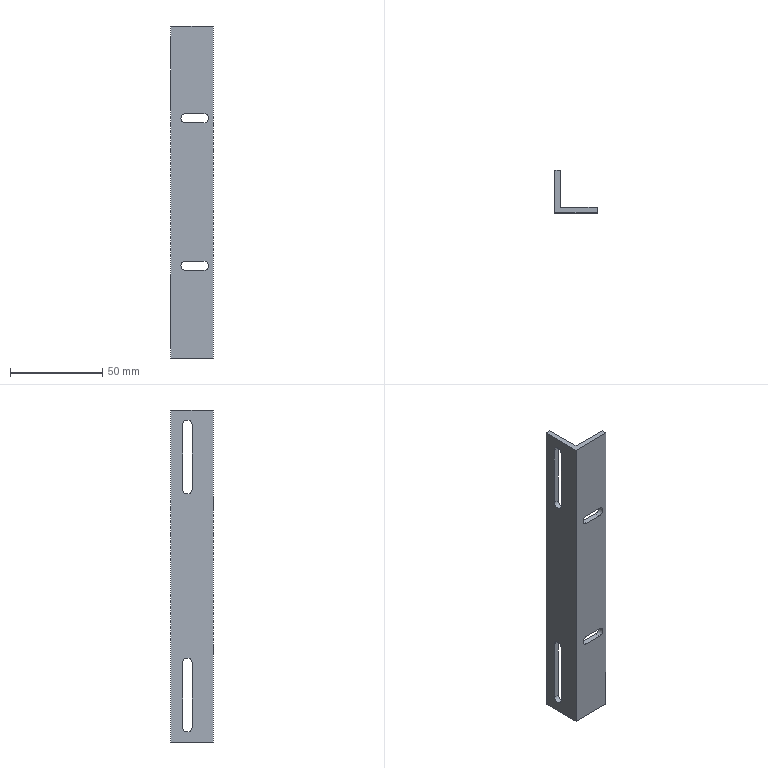Part | SolidWorks | features ICE 2, Extrusion 1, MirrorPattern 1 | 1 solid | 26 faces | box 23 x 23 x 180 mm | volume 21634 mm3 | plane 16 | cylinder 10 | commonest cylinder face diameters 5 x10
STEP:
#1=CARTESIAN_POINT('',(8.,0.,-37.5));
#2=VERTEX_POINT('',#1);
#3=CARTESIAN_POINT('',(5.5,0.,-40.));
#4=VERTEX_POINT('',#3);
#5=CARTESIAN_POINT('',(8.,0.,-40.));
#6=DIRECTION('',(0.,-1.,0.));
#7=DIRECTION('',(-1.,0.,0.));
#8=AXIS2_PLACEMENT_3D('',#5,#6,#7);
#9=CIRCLE('',#8,2.5);
#10=EDGE_CURVE('',#2,#4,#9,.T.);
#11=ORIENTED_EDGE('',*,*,#10,.T.);
#12=CARTESIAN_POINT('',(5.5,3.,-40.));
#13=VERTEX_POINT('',#12);
#14=CARTESIAN_POINT('',(5.5,-0.001,-40.));
#15=DIRECTION('',(0.,1.,0.));
#16=VECTOR('',#15,1000.);
#17=LINE('',#14,#16);
#18=EDGE_CURVE('',#4,#13,#17,.T.);
#19=ORIENTED_EDGE('',*,*,#18,.T.);
#20=CARTESIAN_POINT('',(8.,3.,-37.5));
#21=VERTEX_POINT('',#20);
#22=CARTESIAN_POINT('',(8.,3.,-40.));
#23=DIRECTION('',(0.,1.,0.));
#24=DIRECTION('',(-1.,0.,0.));
#25=AXIS2_PLACEMENT_3D('',#22,#23,#24);
#26=CIRCLE('',#25,2.5);
#27=EDGE_CURVE('',#13,#21,#26,.T.);
#28=ORIENTED_EDGE('',*,*,#27,.T.);
#29=CARTESIAN_POINT('',(8.,-0.001,-37.5));
#30=DIRECTION('',(0.,1.,0.));
#31=VECTOR('',#30,1000.);
#32=LINE('',#29,#31);
#33=EDGE_CURVE('',#2,#21,#32,.T.);
#34=ORIENTED_EDGE('',*,*,#33,.F.);
#35=EDGE_LOOP('',(#11,#19,#28,#34));
#36=FACE_OUTER_BOUND('',#35,.T.);
#37=CARTESIAN_POINT('',(8.,-0.001,-40.));
#38=DIRECTION('',(0.,1.,0.));
#39=DIRECTION('',(-1.,0.,0.));
#40=AXIS2_PLACEMENT_3D('',#37,#38,#39);
#41=CYLINDRICAL_SURFACE('',#40,2.5);
#42=ADVANCED_FACE('',(#36),#41,.F.);
#43=CARTESIAN_POINT('',(8.,0.,42.5));
#44=VERTEX_POINT('',#43);
#45=CARTESIAN_POINT('',(5.5,0.,40.));
#46=VERTEX_POINT('',#45);
#47=CARTESIAN_POINT('',(8.,0.,40.));
#48=DIRECTION('',(0.,-1.,0.));
#49=DIRECTION('',(-1.,0.,0.));
#50=AXIS2_PLACEMENT_3D('',#47,#48,#49);
#51=CIRCLE('',#50,2.5);
#52=EDGE_CURVE('',#44,#46,#51,.T.);
#53=ORIENTED_EDGE('',*,*,#52,.T.);
#54=CARTESIAN_POINT('',(5.5,3.,40.));
#55=VERTEX_POINT('',#54);
#56=CARTESIAN_POINT('',(5.5,-0.001,40.));
#57=DIRECTION('',(0.,1.,0.));
#58=VECTOR('',#57,1000.);
#59=LINE('',#56,#58);
#60=EDGE_CURVE('',#46,#55,#59,.T.);
#61=ORIENTED_EDGE('',*,*,#60,.T.);
#62=CARTESIAN_POINT('',(8.,3.,42.5));
#63=VERTEX_POINT('',#62);
#64=CARTESIAN_POINT('',(8.,3.,40.));
#65=DIRECTION('',(0.,1.,0.));
#66=DIRECTION('',(-1.,0.,0.));
#67=AXIS2_PLACEMENT_3D('',#64,#65,#66);
#68=CIRCLE('',#67,2.5);
#69=EDGE_CURVE('',#55,#63,#68,.T.);
#70=ORIENTED_EDGE('',*,*,#69,.T.);
#71=CARTESIAN_POINT('',(8.,-0.001,42.5));
#72=DIRECTION('',(0.,1.,0.));
#73=VECTOR('',#72,1000.);
#74=LINE('',#71,#73);
#75=EDGE_CURVE('',#44,#63,#74,.T.);
#76=ORIENTED_EDGE('',*,*,#75,.F.);
#77=EDGE_LOOP('',(#53,#61,#70,#76));
#78=FACE_OUTER_BOUND('',#77,.T.);
#79=CARTESIAN_POINT('',(8.,-0.001,40.));
#80=DIRECTION('',(0.,1.,0.));
#81=DIRECTION('',(-1.,0.,0.));
#82=AXIS2_PLACEMENT_3D('',#79,#80,#81);
#83=CYLINDRICAL_SURFACE('',#82,2.5);
#84=ADVANCED_FACE('',(#78),#83,.F.);
#85=CARTESIAN_POINT('',(3.,3.,-90.));
#86=VERTEX_POINT('',#85);
#87=CARTESIAN_POINT('',(3.,23.,-90.));
#88=VERTEX_POINT('',#87);
#89=CARTESIAN_POINT('',(3.,23.,-90.));
#90=DIRECTION('',(0.,1.,0.));
#91=VECTOR('',#90,1000.);
#92=LINE('',#89,#91);
#93=EDGE_CURVE('',#86,#88,#92,.T.);
#94=ORIENTED_EDGE('',*,*,#93,.T.);
#95=CARTESIAN_POINT('',(3.,23.,90.));
#96=VERTEX_POINT('',#95);
#97=CARTESIAN_POINT('',(3.,23.,90.));
#98=DIRECTION('',(0.,0.,-1.));
#99=VECTOR('',#98,1000.);
#100=LINE('',#97,#99);
#101=EDGE_CURVE('',#96,#88,#100,.T.);
#102=ORIENTED_EDGE('',*,*,#101,.F.);
#103=CARTESIAN_POINT('',(3.,3.,90.));
#104=VERTEX_POINT('',#103);
#105=CARTESIAN_POINT('',(3.,23.,90.));
#106=DIRECTION('',(0.,1.,0.));
#107=VECTOR('',#106,1000.);
#108=LINE('',#105,#107);
#109=EDGE_CURVE('',#104,#96,#108,.T.);
#110=ORIENTED_EDGE('',*,*,#109,.F.);
#111=CARTESIAN_POINT('',(3.,3.,90.));
#112=DIRECTION('',(0.,0.,-1.));
#113=VECTOR('',#112,1000.);
#114=LINE('',#111,#113);
#115=EDGE_CURVE('',#104,#86,#114,.T.);
#116=ORIENTED_EDGE('',*,*,#115,.T.);
#117=EDGE_LOOP('',(#94,#102,#110,#116));
#118=FACE_OUTER_BOUND('',#117,.T.);
#119=CARTESIAN_POINT('',(3.,11.5,82.));
#120=VERTEX_POINT('',#119);
#121=CARTESIAN_POINT('',(3.,11.5,47.));
#122=VERTEX_POINT('',#121);
#123=CARTESIAN_POINT('',(3.,11.5,82.));
#124=DIRECTION('',(0.,0.,-1.));
#125=VECTOR('',#124,1000.);
#126=LINE('',#123,#125);
#127=EDGE_CURVE('',#120,#122,#126,.T.);
#128=ORIENTED_EDGE('',*,*,#127,.F.);
#129=CARTESIAN_POINT('',(3.,16.5,82.));
#130=VERTEX_POINT('',#129);
#131=CARTESIAN_POINT('',(3.,14.,82.));
#132=DIRECTION('',(1.,0.,0.));
#133=DIRECTION('',(0.,1.,0.));
#134=AXIS2_PLACEMENT_3D('',#131,#132,#133);
#135=CIRCLE('',#134,2.5);
#136=EDGE_CURVE('',#130,#120,#135,.T.);
#137=ORIENTED_EDGE('',*,*,#136,.F.);
#138=CARTESIAN_POINT('',(3.,16.5,47.));
#139=VERTEX_POINT('',#138);
#140=CARTESIAN_POINT('',(3.,16.5,82.));
#141=DIRECTION('',(0.,0.,1.));
#142=VECTOR('',#141,1000.);
#143=LINE('',#140,#142);
#144=EDGE_CURVE('',#139,#130,#143,.T.);
#145=ORIENTED_EDGE('',*,*,#144,.F.);
#146=CARTESIAN_POINT('',(3.,14.,47.));
#147=DIRECTION('',(1.,0.,0.));
#148=DIRECTION('',(0.,1.,0.));
#149=AXIS2_PLACEMENT_3D('',#146,#147,#148);
#150=CIRCLE('',#149,2.5);
#151=EDGE_CURVE('',#122,#139,#150,.T.);
#152=ORIENTED_EDGE('',*,*,#151,.F.);
#153=EDGE_LOOP('',(#128,#137,#145,#152));
#154=FACE_BOUND('',#153,.T.);
#155=CARTESIAN_POINT('',(3.,16.5,-82.));
#156=VERTEX_POINT('',#155);
#157=CARTESIAN_POINT('',(3.,11.5,-82.));
#158=VERTEX_POINT('',#157);
#159=CARTESIAN_POINT('',(3.,14.,-82.));
#160=DIRECTION('',(-1.,0.,0.));
#161=DIRECTION('',(0.,1.,0.));
#162=AXIS2_PLACEMENT_3D('',#159,#160,#161);
#163=CIRCLE('',#162,2.5);
#164=EDGE_CURVE('',#156,#158,#163,.T.);
#165=ORIENTED_EDGE('',*,*,#164,.T.);
#166=CARTESIAN_POINT('',(3.,11.5,-47.));
#167=VERTEX_POINT('',#166);
#168=CARTESIAN_POINT('',(3.,11.5,-82.));
#169=DIRECTION('',(0.,0.,1.));
#170=VECTOR('',#169,1000.);
#171=LINE('',#168,#170);
#172=EDGE_CURVE('',#158,#167,#171,.T.);
#173=ORIENTED_EDGE('',*,*,#172,.T.);
#174=CARTESIAN_POINT('',(3.,16.5,-47.));
#175=VERTEX_POINT('',#174);
#176=CARTESIAN_POINT('',(3.,14.,-47.));
#177=DIRECTION('',(-1.,0.,0.));
#178=DIRECTION('',(0.,1.,0.));
#179=AXIS2_PLACEMENT_3D('',#176,#177,#178);
#180=CIRCLE('',#179,2.5);
#181=EDGE_CURVE('',#167,#175,#180,.T.);
#182=ORIENTED_EDGE('',*,*,#181,.T.);
#183=CARTESIAN_POINT('',(3.,16.5,-82.));
#184=DIRECTION('',(0.,0.,-1.));
#185=VECTOR('',#184,1000.);
#186=LINE('',#183,#185);
#187=EDGE_CURVE('',#175,#156,#186,.T.);
#188=ORIENTED_EDGE('',*,*,#187,.T.);
#189=EDGE_LOOP('',(#165,#173,#182,#188));
#190=FACE_BOUND('',#189,.T.);
#191=CARTESIAN_POINT('',(3.,23.,90.));
#192=DIRECTION('',(-1.,0.,0.));
#193=DIRECTION('',(0.,-1.,0.));
#194=AXIS2_PLACEMENT_3D('',#191,#192,#193);
#195=PLANE('',#194);
#196=ADVANCED_FACE('',(#118,#154,#190),#195,.F.);
#197=CARTESIAN_POINT('',(0.,23.,-90.));
#198=VERTEX_POINT('',#197);
#199=CARTESIAN_POINT('',(0.,0.,-90.));
#200=VERTEX_POINT('',#199);
#201=CARTESIAN_POINT('',(0.,0.,-90.));
#202=DIRECTION('',(0.,-1.,0.));
#203=VECTOR('',#202,1000.);
#204=LINE('',#201,#203);
#205=EDGE_CURVE('',#198,#200,#204,.T.);
#206=ORIENTED_EDGE('',*,*,#205,.T.);
#207=CARTESIAN_POINT('',(0.,0.,90.));
#208=VERTEX_POINT('',#207);
#209=CARTESIAN_POINT('',(0.,0.,90.));
#210=DIRECTION('',(0.,0.,-1.));
#211=VECTOR('',#210,1000.);
#212=LINE('',#209,#211);
#213=EDGE_CURVE('',#208,#200,#212,.T.);
#214=ORIENTED_EDGE('',*,*,#213,.F.);
#215=CARTESIAN_POINT('',(0.,23.,90.));
#216=VERTEX_POINT('',#215);
#217=CARTESIAN_POINT('',(0.,0.,90.));
#218=DIRECTION('',(0.,-1.,0.));
#219=VECTOR('',#218,1000.);
#220=LINE('',#217,#219);
#221=EDGE_CURVE('',#216,#208,#220,.T.);
#222=ORIENTED_EDGE('',*,*,#221,.F.);
#223=CARTESIAN_POINT('',(0.,23.,90.));
#224=DIRECTION('',(0.,0.,-1.));
#225=VECTOR('',#224,1000.);
#226=LINE('',#223,#225);
#227=EDGE_CURVE('',#216,#198,#226,.T.);
#228=ORIENTED_EDGE('',*,*,#227,.T.);
#229=EDGE_LOOP('',(#206,#214,#222,#228));
#230=FACE_OUTER_BOUND('',#229,.T.);
#231=CARTESIAN_POINT('',(0.,16.5,82.));
#232=VERTEX_POINT('',#231);
#233=CARTESIAN_POINT('',(0.,16.5,47.));
#234=VERTEX_POINT('',#233);
#235=CARTESIAN_POINT('',(0.,16.5,82.));
#236=DIRECTION('',(0.,0.,-1.));
#237=VECTOR('',#236,1000.);
#238=LINE('',#235,#237);
#239=EDGE_CURVE('',#232,#234,#238,.T.);
#240=ORIENTED_EDGE('',*,*,#239,.F.);
#241=CARTESIAN_POINT('',(0.,11.5,82.));
#242=VERTEX_POINT('',#241);
#243=CARTESIAN_POINT('',(0.,14.,82.));
#244=DIRECTION('',(-1.,0.,0.));
#245=DIRECTION('',(0.,1.,0.));
#246=AXIS2_PLACEMENT_3D('',#243,#244,#245);
#247=CIRCLE('',#246,2.5);
#248=EDGE_CURVE('',#242,#232,#247,.T.);
#249=ORIENTED_EDGE('',*,*,#248,.F.);
#250=CARTESIAN_POINT('',(0.,11.5,47.));
#251=VERTEX_POINT('',#250);
#252=CARTESIAN_POINT('',(0.,11.5,82.));
#253=DIRECTION('',(0.,0.,1.));
#254=VECTOR('',#253,1000.);
#255=LINE('',#252,#254);
#256=EDGE_CURVE('',#251,#242,#255,.T.);
#257=ORIENTED_EDGE('',*,*,#256,.F.);
#258=CARTESIAN_POINT('',(0.,14.,47.));
#259=DIRECTION('',(-1.,0.,0.));
#260=DIRECTION('',(0.,1.,0.));
#261=AXIS2_PLACEMENT_3D('',#258,#259,#260);
#262=CIRCLE('',#261,2.5);
#263=EDGE_CURVE('',#234,#251,#262,.T.);
#264=ORIENTED_EDGE('',*,*,#263,.F.);
#265=EDGE_LOOP('',(#240,#249,#257,#264));
#266=FACE_BOUND('',#265,.T.);
#267=CARTESIAN_POINT('',(0.,11.5,-82.));
#268=VERTEX_POINT('',#267);
#269=CARTESIAN_POINT('',(0.,16.5,-82.));
#270=VERTEX_POINT('',#269);
#271=CARTESIAN_POINT('',(0.,14.,-82.));
#272=DIRECTION('',(1.,0.,0.));
#273=DIRECTION('',(0.,1.,0.));
#274=AXIS2_PLACEMENT_3D('',#271,#272,#273);
#275=CIRCLE('',#274,2.5);
#276=EDGE_CURVE('',#268,#270,#275,.T.);
#277=ORIENTED_EDGE('',*,*,#276,.T.);
#278=CARTESIAN_POINT('',(0.,16.5,-47.));
#279=VERTEX_POINT('',#278);
#280=CARTESIAN_POINT('',(0.,16.5,-82.));
#281=DIRECTION('',(0.,0.,1.));
#282=VECTOR('',#281,1000.);
#283=LINE('',#280,#282);
#284=EDGE_CURVE('',#270,#279,#283,.T.);
#285=ORIENTED_EDGE('',*,*,#284,.T.);
#286=CARTESIAN_POINT('',(0.,11.5,-47.));
#287=VERTEX_POINT('',#286);
#288=CARTESIAN_POINT('',(0.,14.,-47.));
#289=DIRECTION('',(1.,0.,0.));
#290=DIRECTION('',(0.,1.,0.));
#291=AXIS2_PLACEMENT_3D('',#288,#289,#290);
#292=CIRCLE('',#291,2.5);
#293=EDGE_CURVE('',#279,#287,#292,.T.);
#294=ORIENTED_EDGE('',*,*,#293,.T.);
#295=CARTESIAN_POINT('',(0.,11.5,-82.));
#296=DIRECTION('',(0.,0.,-1.));
#297=VECTOR('',#296,1000.);
#298=LINE('',#295,#297);
#299=EDGE_CURVE('',#287,#268,#298,.T.);
#300=ORIENTED_EDGE('',*,*,#299,.T.);
#301=EDGE_LOOP('',(#277,#285,#294,#300));
#302=FACE_BOUND('',#301,.T.);
#303=CARTESIAN_POINT('',(0.,0.,90.));
#304=DIRECTION('',(1.,0.,0.));
#305=DIRECTION('',(0.,1.,0.));
#306=AXIS2_PLACEMENT_3D('',#303,#304,#305);
#307=PLANE('',#306);
#308=ADVANCED_FACE('',(#230,#266,#302),#307,.F.);
#309=CARTESIAN_POINT('',(8.,0.,-42.5));
#310=VERTEX_POINT('',#309);
#311=CARTESIAN_POINT('',(18.,0.,-42.5));
#312=VERTEX_POINT('',#311);
#313=CARTESIAN_POINT('',(8.,0.,-42.5));
#314=DIRECTION('',(1.,0.,0.));
#315=VECTOR('',#314,1000.);
#316=LINE('',#313,#315);
#317=EDGE_CURVE('',#310,#312,#316,.T.);
#318=ORIENTED_EDGE('',*,*,#317,.F.);
#319=CARTESIAN_POINT('',(8.,0.,-40.));
#320=DIRECTION('',(0.,-1.,0.));
#321=DIRECTION('',(-1.,0.,0.));
#322=AXIS2_PLACEMENT_3D('',#319,#320,#321);
#323=CIRCLE('',#322,2.5);
#324=EDGE_CURVE('',#4,#310,#323,.T.);
#325=ORIENTED_EDGE('',*,*,#324,.F.);
#326=ORIENTED_EDGE('',*,*,#10,.F.);
#327=CARTESIAN_POINT('',(18.,0.,-37.5));
#328=VERTEX_POINT('',#327);
#329=CARTESIAN_POINT('',(8.,0.,-37.5));
#330=DIRECTION('',(-1.,0.,0.));
#331=VECTOR('',#330,1000.);
#332=LINE('',#329,#331);
#333=EDGE_CURVE('',#328,#2,#332,.T.);
#334=ORIENTED_EDGE('',*,*,#333,.F.);
#335=CARTESIAN_POINT('',(18.,0.,-40.));
#336=DIRECTION('',(0.,-1.,0.));
#337=DIRECTION('',(-1.,0.,0.));
#338=AXIS2_PLACEMENT_3D('',#335,#336,#337);
#339=CIRCLE('',#338,2.5);
#340=EDGE_CURVE('',#312,#328,#339,.T.);
#341=ORIENTED_EDGE('',*,*,#340,.F.);
#342=EDGE_LOOP('',(#318,#325,#326,#334,#341));
#343=FACE_BOUND('',#342,.T.);
#344=CARTESIAN_POINT('',(8.,0.,37.5));
#345=VERTEX_POINT('',#344);
#346=CARTESIAN_POINT('',(18.,0.,37.5));
#347=VERTEX_POINT('',#346);
#348=CARTESIAN_POINT('',(8.,0.,37.5));
#349=DIRECTION('',(1.,0.,0.));
#350=VECTOR('',#349,1000.);
#351=LINE('',#348,#350);
#352=EDGE_CURVE('',#345,#347,#351,.T.);
#353=ORIENTED_EDGE('',*,*,#352,.F.);
#354=CARTESIAN_POINT('',(8.,0.,40.));
#355=DIRECTION('',(0.,-1.,0.));
#356=DIRECTION('',(-1.,0.,0.));
#357=AXIS2_PLACEMENT_3D('',#354,#355,#356);
#358=CIRCLE('',#357,2.5);
#359=EDGE_CURVE('',#46,#345,#358,.T.);
#360=ORIENTED_EDGE('',*,*,#359,.F.);
#361=ORIENTED_EDGE('',*,*,#52,.F.);
#362=CARTESIAN_POINT('',(18.,0.,42.5));
#363=VERTEX_POINT('',#362);
#364=CARTESIAN_POINT('',(8.,0.,42.5));
#365=DIRECTION('',(-1.,0.,0.));
#366=VECTOR('',#365,1000.);
#367=LINE('',#364,#366);
#368=EDGE_CURVE('',#363,#44,#367,.T.);
#369=ORIENTED_EDGE('',*,*,#368,.F.);
#370=CARTESIAN_POINT('',(18.,0.,40.));
#371=DIRECTION('',(0.,-1.,0.));
#372=DIRECTION('',(-1.,0.,0.));
#373=AXIS2_PLACEMENT_3D('',#370,#371,#372);
#374=CIRCLE('',#373,2.5);
#375=EDGE_CURVE('',#347,#363,#374,.T.);
#376=ORIENTED_EDGE('',*,*,#375,.F.);
#377=EDGE_LOOP('',(#353,#360,#361,#369,#376));
#378=FACE_BOUND('',#377,.T.);
#379=CARTESIAN_POINT('',(23.,0.,-90.));
#380=VERTEX_POINT('',#379);
#381=CARTESIAN_POINT('',(23.,0.,-90.));
#382=DIRECTION('',(1.,0.,0.));
#383=VECTOR('',#382,1000.);
#384=LINE('',#381,#383);
#385=EDGE_CURVE('',#200,#380,#384,.T.);
#386=ORIENTED_EDGE('',*,*,#385,.T.);
#387=CARTESIAN_POINT('',(23.,0.,90.));
#388=VERTEX_POINT('',#387);
#389=CARTESIAN_POINT('',(23.,0.,90.));
#390=DIRECTION('',(0.,0.,-1.));
#391=VECTOR('',#390,1000.);
#392=LINE('',#389,#391);
#393=EDGE_CURVE('',#388,#380,#392,.T.);
#394=ORIENTED_EDGE('',*,*,#393,.F.);
#395=CARTESIAN_POINT('',(23.,0.,90.));
#396=DIRECTION('',(1.,0.,0.));
#397=VECTOR('',#396,1000.);
#398=LINE('',#395,#397);
#399=EDGE_CURVE('',#208,#388,#398,.T.);
#400=ORIENTED_EDGE('',*,*,#399,.F.);
#401=ORIENTED_EDGE('',*,*,#213,.T.);
#402=EDGE_LOOP('',(#386,#394,#400,#401));
#403=FACE_OUTER_BOUND('',#402,.T.);
#404=CARTESIAN_POINT('',(23.,0.,90.));
#405=DIRECTION('',(0.,1.,0.));
#406=DIRECTION('',(-1.,0.,0.));
#407=AXIS2_PLACEMENT_3D('',#404,#405,#406);
#408=PLANE('',#407);
#409=ADVANCED_FACE('',(#343,#378,#403),#408,.F.);
#410=CARTESIAN_POINT('',(23.,3.,-90.));
#411=VERTEX_POINT('',#410);
#412=CARTESIAN_POINT('',(23.,3.,-90.));
#413=DIRECTION('',(0.,1.,0.));
#414=VECTOR('',#413,1000.);
#415=LINE('',#412,#414);
#416=EDGE_CURVE('',#380,#411,#415,.T.);
#417=ORIENTED_EDGE('',*,*,#416,.T.);
#418=CARTESIAN_POINT('',(23.,3.,90.));
#419=VERTEX_POINT('',#418);
#420=CARTESIAN_POINT('',(23.,3.,90.));
#421=DIRECTION('',(0.,0.,-1.));
#422=VECTOR('',#421,1000.);
#423=LINE('',#420,#422);
#424=EDGE_CURVE('',#419,#411,#423,.T.);
#425=ORIENTED_EDGE('',*,*,#424,.F.);
#426=CARTESIAN_POINT('',(23.,3.,90.));
#427=DIRECTION('',(0.,1.,0.));
#428=VECTOR('',#427,1000.);
#429=LINE('',#426,#428);
#430=EDGE_CURVE('',#388,#419,#429,.T.);
#431=ORIENTED_EDGE('',*,*,#430,.F.);
#432=ORIENTED_EDGE('',*,*,#393,.T.);
#433=EDGE_LOOP('',(#417,#425,#431,#432));
#434=FACE_OUTER_BOUND('',#433,.T.);
#435=CARTESIAN_POINT('',(23.,3.,90.));
#436=DIRECTION('',(-1.,0.,0.));
#437=DIRECTION('',(0.,0.,1.));
#438=AXIS2_PLACEMENT_3D('',#435,#436,#437);
#439=PLANE('',#438);
#440=ADVANCED_FACE('',(#434),#439,.F.);
#441=CARTESIAN_POINT('',(18.,3.,-37.5));
#442=VERTEX_POINT('',#441);
#443=CARTESIAN_POINT('',(8.,3.,-37.5));
#444=DIRECTION('',(1.,0.,0.));
#445=VECTOR('',#444,1000.);
#446=LINE('',#443,#445);
#447=EDGE_CURVE('',#21,#442,#446,.T.);
#448=ORIENTED_EDGE('',*,*,#447,.F.);
#449=ORIENTED_EDGE('',*,*,#27,.F.);
#450=CARTESIAN_POINT('',(8.,3.,-42.5));
#451=VERTEX_POINT('',#450);
#452=CARTESIAN_POINT('',(8.,3.,-40.));
#453=DIRECTION('',(0.,1.,0.));
#454=DIRECTION('',(-1.,0.,0.));
#455=AXIS2_PLACEMENT_3D('',#452,#453,#454);
#456=CIRCLE('',#455,2.5);
#457=EDGE_CURVE('',#451,#13,#456,.T.);
#458=ORIENTED_EDGE('',*,*,#457,.F.);
#459=CARTESIAN_POINT('',(18.,3.,-42.5));
#460=VERTEX_POINT('',#459);
#461=CARTESIAN_POINT('',(8.,3.,-42.5));
#462=DIRECTION('',(-1.,0.,0.));
#463=VECTOR('',#462,1000.);
#464=LINE('',#461,#463);
#465=EDGE_CURVE('',#460,#451,#464,.T.);
#466=ORIENTED_EDGE('',*,*,#465,.F.);
#467=CARTESIAN_POINT('',(18.,3.,-40.));
#468=DIRECTION('',(0.,1.,0.));
#469=DIRECTION('',(-1.,0.,0.));
#470=AXIS2_PLACEMENT_3D('',#467,#468,#469);
#471=CIRCLE('',#470,2.5);
#472=EDGE_CURVE('',#442,#460,#471,.T.);
#473=ORIENTED_EDGE('',*,*,#472,.F.);
#474=EDGE_LOOP('',(#448,#449,#458,#466,#473));
#475=FACE_BOUND('',#474,.T.);
#476=CARTESIAN_POINT('',(18.,3.,42.5));
#477=VERTEX_POINT('',#476);
#478=CARTESIAN_POINT('',(8.,3.,42.5));
#479=DIRECTION('',(1.,0.,0.));
#480=VECTOR('',#479,1000.);
#481=LINE('',#478,#480);
#482=EDGE_CURVE('',#63,#477,#481,.T.);
#483=ORIENTED_EDGE('',*,*,#482,.F.);
#484=ORIENTED_EDGE('',*,*,#69,.F.);
#485=CARTESIAN_POINT('',(8.,3.,37.5));
#486=VERTEX_POINT('',#485);
#487=CARTESIAN_POINT('',(8.,3.,40.));
#488=DIRECTION('',(0.,1.,0.));
#489=DIRECTION('',(-1.,0.,0.));
#490=AXIS2_PLACEMENT_3D('',#487,#488,#489);
#491=CIRCLE('',#490,2.5);
#492=EDGE_CURVE('',#486,#55,#491,.T.);
#493=ORIENTED_EDGE('',*,*,#492,.F.);
#494=CARTESIAN_POINT('',(18.,3.,37.5));
#495=VERTEX_POINT('',#494);
#496=CARTESIAN_POINT('',(8.,3.,37.5));
#497=DIRECTION('',(-1.,0.,0.));
#498=VECTOR('',#497,1000.);
#499=LINE('',#496,#498);
#500=EDGE_CURVE('',#495,#486,#499,.T.);
#501=ORIENTED_EDGE('',*,*,#500,.F.);
#502=CARTESIAN_POINT('',(18.,3.,40.));
#503=DIRECTION('',(0.,1.,0.));
#504=DIRECTION('',(-1.,0.,0.));
#505=AXIS2_PLACEMENT_3D('',#502,#503,#504);
#506=CIRCLE('',#505,2.5);
#507=EDGE_CURVE('',#477,#495,#506,.T.);
#508=ORIENTED_EDGE('',*,*,#507,.F.);
#509=EDGE_LOOP('',(#483,#484,#493,#501,#508));
#510=FACE_BOUND('',#509,.T.);
#511=CARTESIAN_POINT('',(3.,3.,-90.));
#512=DIRECTION('',(-1.,0.,0.));
#513=VECTOR('',#512,1000.);
#514=LINE('',#511,#513);
#515=EDGE_CURVE('',#411,#86,#514,.T.);
#516=ORIENTED_EDGE('',*,*,#515,.T.);
#517=ORIENTED_EDGE('',*,*,#115,.F.);
#518=CARTESIAN_POINT('',(3.,3.,90.));
#519=DIRECTION('',(-1.,0.,0.));
#520=VECTOR('',#519,1000.);
#521=LINE('',#518,#520);
#522=EDGE_CURVE('',#419,#104,#521,.T.);
#523=ORIENTED_EDGE('',*,*,#522,.F.);
#524=ORIENTED_EDGE('',*,*,#424,.T.);
#525=EDGE_LOOP('',(#516,#517,#523,#524));
#526=FACE_OUTER_BOUND('',#525,.T.);
#527=CARTESIAN_POINT('',(3.,3.,90.));
#528=DIRECTION('',(0.,-1.,0.));
#529=DIRECTION('',(1.,0.,0.));
#530=AXIS2_PLACEMENT_3D('',#527,#528,#529);
#531=PLANE('',#530);
#532=ADVANCED_FACE('',(#475,#510,#526),#531,.F.);
#533=CARTESIAN_POINT('',(0.,23.,-90.));
#534=DIRECTION('',(-1.,0.,0.));
#535=VECTOR('',#534,1000.);
#536=LINE('',#533,#535);
#537=EDGE_CURVE('',#88,#198,#536,.T.);
#538=ORIENTED_EDGE('',*,*,#537,.T.);
#539=ORIENTED_EDGE('',*,*,#227,.F.);
#540=CARTESIAN_POINT('',(0.,23.,90.));
#541=DIRECTION('',(-1.,0.,0.));
#542=VECTOR('',#541,1000.);
#543=LINE('',#540,#542);
#544=EDGE_CURVE('',#96,#216,#543,.T.);
#545=ORIENTED_EDGE('',*,*,#544,.F.);
#546=ORIENTED_EDGE('',*,*,#101,.T.);
#547=EDGE_LOOP('',(#538,#539,#545,#546));
#548=FACE_OUTER_BOUND('',#547,.T.);
#549=CARTESIAN_POINT('',(0.,23.,90.));
#550=DIRECTION('',(0.,-1.,0.));
#551=DIRECTION('',(0.,0.,-1.));
#552=AXIS2_PLACEMENT_3D('',#549,#550,#551);
#553=PLANE('',#552);
#554=ADVANCED_FACE('',(#548),#553,.F.);
#555=ORIENTED_EDGE('',*,*,#399,.T.);
#556=ORIENTED_EDGE('',*,*,#430,.T.);
#557=ORIENTED_EDGE('',*,*,#522,.T.);
#558=ORIENTED_EDGE('',*,*,#109,.T.);
#559=ORIENTED_EDGE('',*,*,#544,.T.);
#560=ORIENTED_EDGE('',*,*,#221,.T.);
#561=EDGE_LOOP('',(#555,#556,#557,#558,#559,#560));
#562=FACE_OUTER_BOUND('',#561,.T.);
#563=CARTESIAN_POINT('',(0.,0.,90.));
#564=DIRECTION('',(0.,0.,-1.));
#565=DIRECTION('',(-1.,0.,0.));
#566=AXIS2_PLACEMENT_3D('',#563,#564,#565);
#567=PLANE('',#566);
#568=ADVANCED_FACE('',(#562),#567,.F.);
#569=ORIENTED_EDGE('',*,*,#385,.F.);
#570=ORIENTED_EDGE('',*,*,#205,.F.);
#571=ORIENTED_EDGE('',*,*,#537,.F.);
#572=ORIENTED_EDGE('',*,*,#93,.F.);
#573=ORIENTED_EDGE('',*,*,#515,.F.);
#574=ORIENTED_EDGE('',*,*,#416,.F.);
#575=EDGE_LOOP('',(#569,#570,#571,#572,#573,#574));
#576=FACE_OUTER_BOUND('',#575,.T.);
#577=CARTESIAN_POINT('',(0.,0.,-90.));
#578=DIRECTION('',(0.,0.,-1.));
#579=DIRECTION('',(-1.,0.,0.));
#580=AXIS2_PLACEMENT_3D('',#577,#578,#579);
#581=PLANE('',#580);
#582=ADVANCED_FACE('',(#576),#581,.T.);
#583=ORIENTED_EDGE('',*,*,#248,.T.);
#584=CARTESIAN_POINT('',(-0.001,16.5,82.));
#585=DIRECTION('',(1.,0.,0.));
#586=VECTOR('',#585,1000.);
#587=LINE('',#584,#586);
#588=EDGE_CURVE('',#232,#130,#587,.T.);
#589=ORIENTED_EDGE('',*,*,#588,.T.);
#590=ORIENTED_EDGE('',*,*,#136,.T.);
#591=CARTESIAN_POINT('',(-0.001,11.5,82.));
#592=DIRECTION('',(1.,0.,0.));
#593=VECTOR('',#592,1000.);
#594=LINE('',#591,#593);
#595=EDGE_CURVE('',#242,#120,#594,.T.);
#596=ORIENTED_EDGE('',*,*,#595,.F.);
#597=EDGE_LOOP('',(#583,#589,#590,#596));
#598=FACE_OUTER_BOUND('',#597,.T.);
#599=CARTESIAN_POINT('',(-0.001,14.,82.));
#600=DIRECTION('',(1.,0.,0.));
#601=DIRECTION('',(0.,1.,0.));
#602=AXIS2_PLACEMENT_3D('',#599,#600,#601);
#603=CYLINDRICAL_SURFACE('',#602,2.5);
#604=ADVANCED_FACE('',(#598),#603,.F.);
#605=ORIENTED_EDGE('',*,*,#239,.T.);
#606=CARTESIAN_POINT('',(-0.001,16.5,47.));
#607=DIRECTION('',(1.,0.,0.));
#608=VECTOR('',#607,1000.);
#609=LINE('',#606,#608);
#610=EDGE_CURVE('',#234,#139,#609,.T.);
#611=ORIENTED_EDGE('',*,*,#610,.T.);
#612=ORIENTED_EDGE('',*,*,#144,.T.);
#613=ORIENTED_EDGE('',*,*,#588,.F.);
#614=EDGE_LOOP('',(#605,#611,#612,#613));
#615=FACE_OUTER_BOUND('',#614,.T.);
#616=CARTESIAN_POINT('',(-0.001,16.5,82.));
#617=DIRECTION('',(0.,1.,0.));
#618=DIRECTION('',(-1.,0.,0.));
#619=AXIS2_PLACEMENT_3D('',#616,#617,#618);
#620=PLANE('',#619);
#621=ADVANCED_FACE('',(#615),#620,.F.);
#622=ORIENTED_EDGE('',*,*,#263,.T.);
#623=CARTESIAN_POINT('',(-0.001,11.5,47.));
#624=DIRECTION('',(1.,0.,0.));
#625=VECTOR('',#624,1000.);
#626=LINE('',#623,#625);
#627=EDGE_CURVE('',#251,#122,#626,.T.);
#628=ORIENTED_EDGE('',*,*,#627,.T.);
#629=ORIENTED_EDGE('',*,*,#151,.T.);
#630=ORIENTED_EDGE('',*,*,#610,.F.);
#631=EDGE_LOOP('',(#622,#628,#629,#630));
#632=FACE_OUTER_BOUND('',#631,.T.);
#633=CARTESIAN_POINT('',(-0.001,14.,47.));
#634=DIRECTION('',(1.,0.,0.));
#635=DIRECTION('',(0.,1.,0.));
#636=AXIS2_PLACEMENT_3D('',#633,#634,#635);
#637=CYLINDRICAL_SURFACE('',#636,2.5);
#638=ADVANCED_FACE('',(#632),#637,.F.);
#639=ORIENTED_EDGE('',*,*,#256,.T.);
#640=ORIENTED_EDGE('',*,*,#595,.T.);
#641=ORIENTED_EDGE('',*,*,#127,.T.);
#642=ORIENTED_EDGE('',*,*,#627,.F.);
#643=EDGE_LOOP('',(#639,#640,#641,#642));
#644=FACE_OUTER_BOUND('',#643,.T.);
#645=CARTESIAN_POINT('',(-0.001,11.5,82.));
#646=DIRECTION('',(0.,-1.,0.));
#647=DIRECTION('',(1.,0.,0.));
#648=AXIS2_PLACEMENT_3D('',#645,#646,#647);
#649=PLANE('',#648);
#650=ADVANCED_FACE('',(#644),#649,.F.);
#651=CARTESIAN_POINT('',(-0.001,11.5,-82.));
#652=DIRECTION('',(1.,0.,0.));
#653=VECTOR('',#652,1000.);
#654=LINE('',#651,#653);
#655=EDGE_CURVE('',#268,#158,#654,.T.);
#656=ORIENTED_EDGE('',*,*,#655,.T.);
#657=ORIENTED_EDGE('',*,*,#164,.F.);
#658=CARTESIAN_POINT('',(-0.001,16.5,-82.));
#659=DIRECTION('',(1.,0.,0.));
#660=VECTOR('',#659,1000.);
#661=LINE('',#658,#660);
#662=EDGE_CURVE('',#270,#156,#661,.T.);
#663=ORIENTED_EDGE('',*,*,#662,.F.);
#664=ORIENTED_EDGE('',*,*,#276,.F.);
#665=EDGE_LOOP('',(#656,#657,#663,#664));
#666=FACE_OUTER_BOUND('',#665,.T.);
#667=CARTESIAN_POINT('',(-0.001,14.,-82.));
#668=DIRECTION('',(1.,0.,0.));
#669=DIRECTION('',(0.,1.,0.));
#670=AXIS2_PLACEMENT_3D('',#667,#668,#669);
#671=CYLINDRICAL_SURFACE('',#670,2.5);
#672=ADVANCED_FACE('',(#666),#671,.F.);
#673=CARTESIAN_POINT('',(-0.001,11.5,-47.));
#674=DIRECTION('',(1.,0.,0.));
#675=VECTOR('',#674,1000.);
#676=LINE('',#673,#675);
#677=EDGE_CURVE('',#287,#167,#676,.T.);
#678=ORIENTED_EDGE('',*,*,#677,.T.);
#679=ORIENTED_EDGE('',*,*,#172,.F.);
#680=ORIENTED_EDGE('',*,*,#655,.F.);
#681=ORIENTED_EDGE('',*,*,#299,.F.);
#682=EDGE_LOOP('',(#678,#679,#680,#681));
#683=FACE_OUTER_BOUND('',#682,.T.);
#684=CARTESIAN_POINT('',(-0.001,11.5,-82.));
#685=DIRECTION('',(0.,1.,0.));
#686=DIRECTION('',(-1.,0.,0.));
#687=AXIS2_PLACEMENT_3D('',#684,#685,#686);
#688=PLANE('',#687);
#689=ADVANCED_FACE('',(#683),#688,.T.);
#690=CARTESIAN_POINT('',(-0.001,16.5,-47.));
#691=DIRECTION('',(1.,0.,0.));
#692=VECTOR('',#691,1000.);
#693=LINE('',#690,#692);
#694=EDGE_CURVE('',#279,#175,#693,.T.);
#695=ORIENTED_EDGE('',*,*,#694,.T.);
#696=ORIENTED_EDGE('',*,*,#181,.F.);
#697=ORIENTED_EDGE('',*,*,#677,.F.);
#698=ORIENTED_EDGE('',*,*,#293,.F.);
#699=EDGE_LOOP('',(#695,#696,#697,#698));
#700=FACE_OUTER_BOUND('',#699,.T.);
#701=CARTESIAN_POINT('',(-0.001,14.,-47.));
#702=DIRECTION('',(1.,0.,0.));
#703=DIRECTION('',(0.,1.,0.));
#704=AXIS2_PLACEMENT_3D('',#701,#702,#703);
#705=CYLINDRICAL_SURFACE('',#704,2.5);
#706=ADVANCED_FACE('',(#700),#705,.F.);
#707=ORIENTED_EDGE('',*,*,#662,.T.);
#708=ORIENTED_EDGE('',*,*,#187,.F.);
#709=ORIENTED_EDGE('',*,*,#694,.F.);
#710=ORIENTED_EDGE('',*,*,#284,.F.);
#711=EDGE_LOOP('',(#707,#708,#709,#710));
#712=FACE_OUTER_BOUND('',#711,.T.);
#713=CARTESIAN_POINT('',(-0.001,16.5,-82.));
#714=DIRECTION('',(0.,-1.,0.));
#715=DIRECTION('',(1.,0.,0.));
#716=AXIS2_PLACEMENT_3D('',#713,#714,#715);
#717=PLANE('',#716);
#718=ADVANCED_FACE('',(#712),#717,.T.);
#719=ORIENTED_EDGE('',*,*,#60,.F.);
#720=ORIENTED_EDGE('',*,*,#359,.T.);
#721=CARTESIAN_POINT('',(8.,-0.001,37.5));
#722=DIRECTION('',(0.,1.,0.));
#723=VECTOR('',#722,1000.);
#724=LINE('',#721,#723);
#725=EDGE_CURVE('',#345,#486,#724,.T.);
#726=ORIENTED_EDGE('',*,*,#725,.T.);
#727=ORIENTED_EDGE('',*,*,#492,.T.);
#728=EDGE_LOOP('',(#719,#720,#726,#727));
#729=FACE_OUTER_BOUND('',#728,.T.);
#730=CARTESIAN_POINT('',(8.,-0.001,40.));
#731=DIRECTION('',(0.,1.,0.));
#732=DIRECTION('',(-1.,0.,0.));
#733=AXIS2_PLACEMENT_3D('',#730,#731,#732);
#734=CYLINDRICAL_SURFACE('',#733,2.5);
#735=ADVANCED_FACE('',(#729),#734,.F.);
#736=ORIENTED_EDGE('',*,*,#352,.T.);
#737=CARTESIAN_POINT('',(18.,-0.001,37.5));
#738=DIRECTION('',(0.,1.,0.));
#739=VECTOR('',#738,1000.);
#740=LINE('',#737,#739);
#741=EDGE_CURVE('',#347,#495,#740,.T.);
#742=ORIENTED_EDGE('',*,*,#741,.T.);
#743=ORIENTED_EDGE('',*,*,#500,.T.);
#744=ORIENTED_EDGE('',*,*,#725,.F.);
#745=EDGE_LOOP('',(#736,#742,#743,#744));
#746=FACE_OUTER_BOUND('',#745,.T.);
#747=CARTESIAN_POINT('',(8.,-0.001,37.5));
#748=DIRECTION('',(0.,0.,-1.));
#749=DIRECTION('',(-1.,0.,0.));
#750=AXIS2_PLACEMENT_3D('',#747,#748,#749);
#751=PLANE('',#750);
#752=ADVANCED_FACE('',(#746),#751,.F.);
#753=ORIENTED_EDGE('',*,*,#375,.T.);
#754=CARTESIAN_POINT('',(18.,-0.001,42.5));
#755=DIRECTION('',(0.,1.,0.));
#756=VECTOR('',#755,1000.);
#757=LINE('',#754,#756);
#758=EDGE_CURVE('',#363,#477,#757,.T.);
#759=ORIENTED_EDGE('',*,*,#758,.T.);
#760=ORIENTED_EDGE('',*,*,#507,.T.);
#761=ORIENTED_EDGE('',*,*,#741,.F.);
#762=EDGE_LOOP('',(#753,#759,#760,#761));
#763=FACE_OUTER_BOUND('',#762,.T.);
#764=CARTESIAN_POINT('',(18.,-0.001,40.));
#765=DIRECTION('',(0.,1.,0.));
#766=DIRECTION('',(-1.,0.,0.));
#767=AXIS2_PLACEMENT_3D('',#764,#765,#766);
#768=CYLINDRICAL_SURFACE('',#767,2.5);
#769=ADVANCED_FACE('',(#763),#768,.F.);
#770=ORIENTED_EDGE('',*,*,#368,.T.);
#771=ORIENTED_EDGE('',*,*,#75,.T.);
#772=ORIENTED_EDGE('',*,*,#482,.T.);
#773=ORIENTED_EDGE('',*,*,#758,.F.);
#774=EDGE_LOOP('',(#770,#771,#772,#773));
#775=FACE_OUTER_BOUND('',#774,.T.);
#776=CARTESIAN_POINT('',(8.,-0.001,42.5));
#777=DIRECTION('',(0.,0.,1.));
#778=DIRECTION('',(1.,0.,0.));
#779=AXIS2_PLACEMENT_3D('',#776,#777,#778);
#780=PLANE('',#779);
#781=ADVANCED_FACE('',(#775),#780,.F.);
#782=ORIENTED_EDGE('',*,*,#18,.F.);
#783=ORIENTED_EDGE('',*,*,#324,.T.);
#784=CARTESIAN_POINT('',(8.,-0.001,-42.5));
#785=DIRECTION('',(0.,1.,0.));
#786=VECTOR('',#785,1000.);
#787=LINE('',#784,#786);
#788=EDGE_CURVE('',#310,#451,#787,.T.);
#789=ORIENTED_EDGE('',*,*,#788,.T.);
#790=ORIENTED_EDGE('',*,*,#457,.T.);
#791=EDGE_LOOP('',(#782,#783,#789,#790));
#792=FACE_OUTER_BOUND('',#791,.T.);
#793=CARTESIAN_POINT('',(8.,-0.001,-40.));
#794=DIRECTION('',(0.,1.,0.));
#795=DIRECTION('',(-1.,0.,0.));
#796=AXIS2_PLACEMENT_3D('',#793,#794,#795);
#797=CYLINDRICAL_SURFACE('',#796,2.5);
#798=ADVANCED_FACE('',(#792),#797,.F.);
#799=ORIENTED_EDGE('',*,*,#317,.T.);
#800=CARTESIAN_POINT('',(18.,-0.001,-42.5));
#801=DIRECTION('',(0.,1.,0.));
#802=VECTOR('',#801,1000.);
#803=LINE('',#800,#802);
#804=EDGE_CURVE('',#312,#460,#803,.T.);
#805=ORIENTED_EDGE('',*,*,#804,.T.);
#806=ORIENTED_EDGE('',*,*,#465,.T.);
#807=ORIENTED_EDGE('',*,*,#788,.F.);
#808=EDGE_LOOP('',(#799,#805,#806,#807));
#809=FACE_OUTER_BOUND('',#808,.T.);
#810=CARTESIAN_POINT('',(8.,-0.001,-42.5));
#811=DIRECTION('',(0.,0.,-1.));
#812=DIRECTION('',(-1.,0.,0.));
#813=AXIS2_PLACEMENT_3D('',#810,#811,#812);
#814=PLANE('',#813);
#815=ADVANCED_FACE('',(#809),#814,.F.);
#816=ORIENTED_EDGE('',*,*,#340,.T.);
#817=CARTESIAN_POINT('',(18.,-0.001,-37.5));
#818=DIRECTION('',(0.,1.,0.));
#819=VECTOR('',#818,1000.);
#820=LINE('',#817,#819);
#821=EDGE_CURVE('',#328,#442,#820,.T.);
#822=ORIENTED_EDGE('',*,*,#821,.T.);
#823=ORIENTED_EDGE('',*,*,#472,.T.);
#824=ORIENTED_EDGE('',*,*,#804,.F.);
#825=EDGE_LOOP('',(#816,#822,#823,#824));
#826=FACE_OUTER_BOUND('',#825,.T.);
#827=CARTESIAN_POINT('',(18.,-0.001,-40.));
#828=DIRECTION('',(0.,1.,0.));
#829=DIRECTION('',(-1.,0.,0.));
#830=AXIS2_PLACEMENT_3D('',#827,#828,#829);
#831=CYLINDRICAL_SURFACE('',#830,2.5);
#832=ADVANCED_FACE('',(#826),#831,.F.);
#833=ORIENTED_EDGE('',*,*,#333,.T.);
#834=ORIENTED_EDGE('',*,*,#33,.T.);
#835=ORIENTED_EDGE('',*,*,#447,.T.);
#836=ORIENTED_EDGE('',*,*,#821,.F.);
#837=EDGE_LOOP('',(#833,#834,#835,#836));
#838=FACE_OUTER_BOUND('',#837,.T.);
#839=CARTESIAN_POINT('',(8.,-0.001,-37.5));
#840=DIRECTION('',(0.,0.,1.));
#841=DIRECTION('',(1.,0.,0.));
#842=AXIS2_PLACEMENT_3D('',#839,#840,#841);
#843=PLANE('',#842);
#844=ADVANCED_FACE('',(#838),#843,.F.);
#845=CLOSED_SHELL('',(#42,#84,#196,#308,#409,#440,#532,#554,#568,#582,#604,#621,#638,#650,#672,#689,#706,#718,#735,#752,#769,#781,#798,#815,#832,#844));
#846=MANIFOLD_SOLID_BREP('',#845);
#847=CARTESIAN_POINT('',(0.,0.,0.));
#848=DIRECTION('',(0.,0.,1.));
#849=DIRECTION('',(1.,0.,0.));
#850=AXIS2_PLACEMENT_3D('',#847,#848,#849);
#851=(LENGTH_UNIT()NAMED_UNIT(*)SI_UNIT(.MILLI.,.METRE.));
#852=UNCERTAINTY_MEASURE_WITH_UNIT(LENGTH_MEASURE(0.00001),#851,'','');
#853=(NAMED_UNIT(*)PLANE_ANGLE_UNIT()SI_UNIT($,.RADIAN.));
#854=(NAMED_UNIT(*)SI_UNIT($,.STERADIAN.)SOLID_ANGLE_UNIT());
#855=(GEOMETRIC_REPRESENTATION_CONTEXT(3)GLOBAL_UNCERTAINTY_ASSIGNED_CONTEXT((#852))GLOBAL_UNIT_ASSIGNED_CONTEXT((#851,#853,#854))REPRESENTATION_CONTEXT('',''));
#856=ADVANCED_BREP_SHAPE_REPRESENTATION('',(#846,#850),#855);